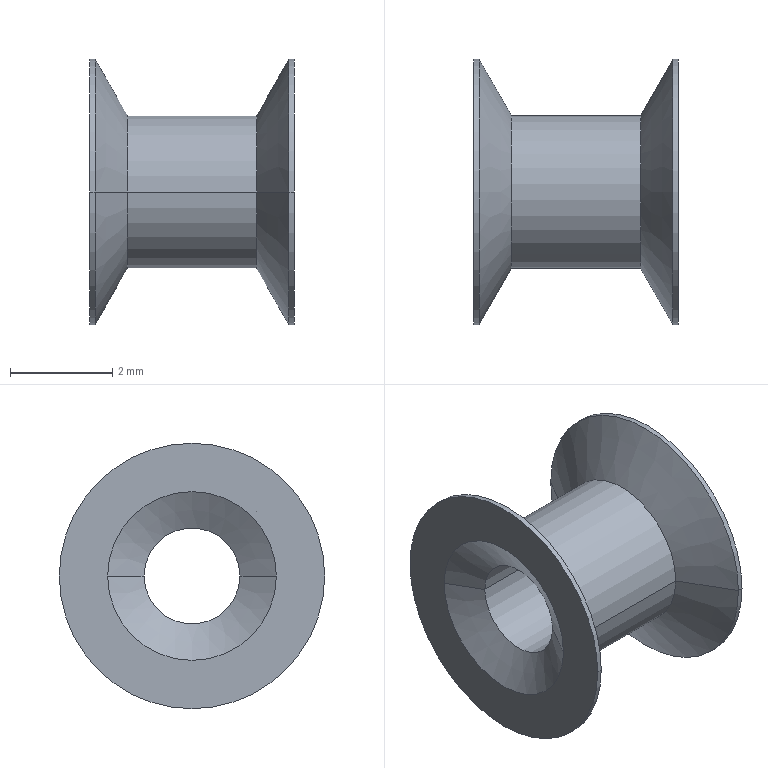Part | NX | features solid 2 | 1 solid | 18 faces | box 4 x 5.2 x 5.2 mm | volume 26.025 mm3 | cylinder 8 | cone 8 | plane 2 | commonest cylinder face diameters 5.2 x4 1.88 x2 3 x2
STEP:
#1=CARTESIAN_POINT('',(13.5,2156.1,-1040.27));
#2=VERTEX_POINT('',#1);
#3=CARTESIAN_POINT('',(13.5,2150.9,-1040.27));
#4=VERTEX_POINT('',#3);
#5=CARTESIAN_POINT('',(13.5,2153.5,-1040.27));
#6=DIRECTION('',(1.,0.,0.));
#7=DIRECTION('',(0.,1.,0.));
#8=AXIS2_PLACEMENT_3D('',#5,#6,#7);
#9=CIRCLE('',#8,2.6);
#10=EDGE_CURVE('',#2,#4,#9,.T.);
#11=ORIENTED_EDGE('',*,*,#10,.F.);
#12=CARTESIAN_POINT('',(13.5,2153.5,-1040.27));
#13=DIRECTION('',(1.,0.,0.));
#14=DIRECTION('',(0.,-1.,0.));
#15=AXIS2_PLACEMENT_3D('',#12,#13,#14);
#16=CIRCLE('',#15,2.6);
#17=EDGE_CURVE('',#4,#2,#16,.T.);
#18=ORIENTED_EDGE('',*,*,#17,.F.);
#19=EDGE_LOOP('',(#11,#18));
#20=FACE_BOUND('',#19,.T.);
#21=CARTESIAN_POINT('',(13.5,2155.153,-1040.27));
#22=VERTEX_POINT('',#21);
#23=CARTESIAN_POINT('',(13.5,2151.847,-1040.27));
#24=VERTEX_POINT('',#23);
#25=CARTESIAN_POINT('',(13.5,2153.5,-1040.27));
#26=DIRECTION('',(-1.,0.,0.));
#27=DIRECTION('',(0.,1.,0.));
#28=AXIS2_PLACEMENT_3D('',#25,#26,#27);
#29=CIRCLE('',#28,1.653);
#30=EDGE_CURVE('',#22,#24,#29,.T.);
#31=ORIENTED_EDGE('',*,*,#30,.F.);
#32=CARTESIAN_POINT('',(13.5,2153.5,-1040.27));
#33=DIRECTION('',(-1.,0.,0.));
#34=DIRECTION('',(0.,-1.,0.));
#35=AXIS2_PLACEMENT_3D('',#32,#33,#34);
#36=CIRCLE('',#35,1.653);
#37=EDGE_CURVE('',#24,#22,#36,.T.);
#38=ORIENTED_EDGE('',*,*,#37,.F.);
#39=EDGE_LOOP('',(#31,#38));
#40=FACE_BOUND('',#39,.T.);
#41=CARTESIAN_POINT('',(13.5,2153.5,-1040.27));
#42=DIRECTION('',(-1.,0.,0.));
#43=DIRECTION('',(0.,-1.,0.));
#44=AXIS2_PLACEMENT_3D('',#41,#42,#43);
#45=PLANE('',#44);
#46=ADVANCED_FACE('',(#20,#40),#45,.T.);
#47=ORIENTED_EDGE('',*,*,#17,.T.);
#48=CARTESIAN_POINT('',(13.6,2156.1,-1040.27));
#49=VERTEX_POINT('',#48);
#50=CARTESIAN_POINT('',(13.5,2156.1,-1040.27));
#51=DIRECTION('',(1.,0.,0.));
#52=VECTOR('',#51,1000.);
#53=LINE('',#50,#52);
#54=EDGE_CURVE('',#2,#49,#53,.T.);
#55=ORIENTED_EDGE('',*,*,#54,.T.);
#56=CARTESIAN_POINT('',(13.6,2150.9,-1040.27));
#57=VERTEX_POINT('',#56);
#58=CARTESIAN_POINT('',(13.6,2153.5,-1040.27));
#59=DIRECTION('',(-1.,0.,0.));
#60=DIRECTION('',(0.,1.,0.));
#61=AXIS2_PLACEMENT_3D('',#58,#59,#60);
#62=CIRCLE('',#61,2.6);
#63=EDGE_CURVE('',#49,#57,#62,.T.);
#64=ORIENTED_EDGE('',*,*,#63,.T.);
#65=CARTESIAN_POINT('',(13.5,2150.9,-1040.27));
#66=DIRECTION('',(1.,0.,0.));
#67=VECTOR('',#66,1000.);
#68=LINE('',#65,#67);
#69=EDGE_CURVE('',#57,#4,#68,.F.);
#70=ORIENTED_EDGE('',*,*,#69,.T.);
#71=EDGE_LOOP('',(#47,#55,#64,#70));
#72=FACE_BOUND('',#71,.T.);
#73=CARTESIAN_POINT('',(17.7,2153.5,-1040.27));
#74=DIRECTION('',(-1.,0.,0.));
#75=DIRECTION('',(0.,-1.,0.));
#76=AXIS2_PLACEMENT_3D('',#73,#74,#75);
#77=CYLINDRICAL_SURFACE('',#76,2.6);
#78=ADVANCED_FACE('',(#72),#77,.T.);
#79=CARTESIAN_POINT('',(13.6,2153.5,-1040.27));
#80=DIRECTION('',(-1.,0.,0.));
#81=DIRECTION('',(0.,-1.,0.));
#82=AXIS2_PLACEMENT_3D('',#79,#80,#81);
#83=CIRCLE('',#82,2.6);
#84=EDGE_CURVE('',#57,#49,#83,.T.);
#85=ORIENTED_EDGE('',*,*,#84,.T.);
#86=ORIENTED_EDGE('',*,*,#54,.F.);
#87=ORIENTED_EDGE('',*,*,#10,.T.);
#88=ORIENTED_EDGE('',*,*,#69,.F.);
#89=EDGE_LOOP('',(#85,#86,#87,#88));
#90=FACE_BOUND('',#89,.T.);
#91=CARTESIAN_POINT('',(17.7,2153.5,-1040.27));
#92=DIRECTION('',(-1.,0.,0.));
#93=DIRECTION('',(0.,-1.,0.));
#94=AXIS2_PLACEMENT_3D('',#91,#92,#93);
#95=CYLINDRICAL_SURFACE('',#94,2.6);
#96=ADVANCED_FACE('',(#90),#95,.T.);
#97=CARTESIAN_POINT('',(14.235,2155.,-1040.27));
#98=VERTEX_POINT('',#97);
#99=CARTESIAN_POINT('',(14.235,2152.,-1040.27));
#100=VERTEX_POINT('',#99);
#101=CARTESIAN_POINT('',(14.235,2153.5,-1040.27));
#102=DIRECTION('',(1.,0.,0.));
#103=DIRECTION('',(0.,1.,0.));
#104=AXIS2_PLACEMENT_3D('',#101,#102,#103);
#105=CIRCLE('',#104,1.5);
#106=EDGE_CURVE('',#98,#100,#105,.T.);
#107=ORIENTED_EDGE('',*,*,#106,.F.);
#108=CARTESIAN_POINT('',(13.6,2156.1,-1040.27));
#109=DIRECTION('',(0.5,-0.866,0.));
#110=VECTOR('',#109,1000.);
#111=LINE('',#108,#110);
#112=EDGE_CURVE('',#49,#98,#111,.T.);
#113=ORIENTED_EDGE('',*,*,#112,.F.);
#114=ORIENTED_EDGE('',*,*,#84,.F.);
#115=CARTESIAN_POINT('',(13.6,2150.9,-1040.27));
#116=DIRECTION('',(0.5,0.866,0.));
#117=VECTOR('',#116,1000.);
#118=LINE('',#115,#117);
#119=EDGE_CURVE('',#100,#57,#118,.F.);
#120=ORIENTED_EDGE('',*,*,#119,.F.);
#121=EDGE_LOOP('',(#107,#113,#114,#120));
#122=FACE_BOUND('',#121,.T.);
#123=CARTESIAN_POINT('',(13.918,2153.5,-1040.27));
#124=DIRECTION('',(-1.,0.,0.));
#125=DIRECTION('',(0.,-1.,0.));
#126=AXIS2_PLACEMENT_3D('',#123,#124,#125);
#127=CONICAL_SURFACE('',#126,2.05,1.047);
#128=ADVANCED_FACE('',(#122),#127,.T.);
#129=ORIENTED_EDGE('',*,*,#63,.F.);
#130=ORIENTED_EDGE('',*,*,#112,.T.);
#131=CARTESIAN_POINT('',(14.235,2153.5,-1040.27));
#132=DIRECTION('',(1.,0.,0.));
#133=DIRECTION('',(0.,-1.,0.));
#134=AXIS2_PLACEMENT_3D('',#131,#132,#133);
#135=CIRCLE('',#134,1.5);
#136=EDGE_CURVE('',#100,#98,#135,.T.);
#137=ORIENTED_EDGE('',*,*,#136,.F.);
#138=ORIENTED_EDGE('',*,*,#119,.T.);
#139=EDGE_LOOP('',(#129,#130,#137,#138));
#140=FACE_BOUND('',#139,.T.);
#141=CARTESIAN_POINT('',(13.918,2153.5,-1040.27));
#142=DIRECTION('',(-1.,0.,0.));
#143=DIRECTION('',(0.,-1.,0.));
#144=AXIS2_PLACEMENT_3D('',#141,#142,#143);
#145=CONICAL_SURFACE('',#144,2.05,1.047);
#146=ADVANCED_FACE('',(#140),#145,.T.);
#147=ORIENTED_EDGE('',*,*,#136,.T.);
#148=CARTESIAN_POINT('',(16.765,2155.,-1040.27));
#149=VERTEX_POINT('',#148);
#150=CARTESIAN_POINT('',(14.235,2155.,-1040.27));
#151=DIRECTION('',(1.,0.,0.));
#152=VECTOR('',#151,1000.);
#153=LINE('',#150,#152);
#154=EDGE_CURVE('',#98,#149,#153,.T.);
#155=ORIENTED_EDGE('',*,*,#154,.T.);
#156=CARTESIAN_POINT('',(16.765,2152.,-1040.27));
#157=VERTEX_POINT('',#156);
#158=CARTESIAN_POINT('',(16.765,2153.5,-1040.27));
#159=DIRECTION('',(-1.,0.,0.));
#160=DIRECTION('',(0.,1.,0.));
#161=AXIS2_PLACEMENT_3D('',#158,#159,#160);
#162=CIRCLE('',#161,1.5);
#163=EDGE_CURVE('',#149,#157,#162,.T.);
#164=ORIENTED_EDGE('',*,*,#163,.T.);
#165=CARTESIAN_POINT('',(14.235,2152.,-1040.27));
#166=DIRECTION('',(1.,0.,0.));
#167=VECTOR('',#166,1000.);
#168=LINE('',#165,#167);
#169=EDGE_CURVE('',#157,#100,#168,.F.);
#170=ORIENTED_EDGE('',*,*,#169,.T.);
#171=EDGE_LOOP('',(#147,#155,#164,#170));
#172=FACE_BOUND('',#171,.T.);
#173=CARTESIAN_POINT('',(17.7,2153.5,-1040.27));
#174=DIRECTION('',(-1.,0.,0.));
#175=DIRECTION('',(0.,-1.,0.));
#176=AXIS2_PLACEMENT_3D('',#173,#174,#175);
#177=CYLINDRICAL_SURFACE('',#176,1.5);
#178=ADVANCED_FACE('',(#172),#177,.T.);
#179=CARTESIAN_POINT('',(16.765,2153.5,-1040.27));
#180=DIRECTION('',(-1.,0.,0.));
#181=DIRECTION('',(0.,-1.,0.));
#182=AXIS2_PLACEMENT_3D('',#179,#180,#181);
#183=CIRCLE('',#182,1.5);
#184=EDGE_CURVE('',#157,#149,#183,.T.);
#185=ORIENTED_EDGE('',*,*,#184,.T.);
#186=ORIENTED_EDGE('',*,*,#154,.F.);
#187=ORIENTED_EDGE('',*,*,#106,.T.);
#188=ORIENTED_EDGE('',*,*,#169,.F.);
#189=EDGE_LOOP('',(#185,#186,#187,#188));
#190=FACE_BOUND('',#189,.T.);
#191=CARTESIAN_POINT('',(17.7,2153.5,-1040.27));
#192=DIRECTION('',(-1.,0.,0.));
#193=DIRECTION('',(0.,-1.,0.));
#194=AXIS2_PLACEMENT_3D('',#191,#192,#193);
#195=CYLINDRICAL_SURFACE('',#194,1.5);
#196=ADVANCED_FACE('',(#190),#195,.T.);
#197=CARTESIAN_POINT('',(17.4,2156.1,-1040.27));
#198=VERTEX_POINT('',#197);
#199=CARTESIAN_POINT('',(17.4,2150.9,-1040.27));
#200=VERTEX_POINT('',#199);
#201=CARTESIAN_POINT('',(17.4,2153.5,-1040.27));
#202=DIRECTION('',(1.,0.,0.));
#203=DIRECTION('',(0.,1.,0.));
#204=AXIS2_PLACEMENT_3D('',#201,#202,#203);
#205=CIRCLE('',#204,2.6);
#206=EDGE_CURVE('',#198,#200,#205,.T.);
#207=ORIENTED_EDGE('',*,*,#206,.F.);
#208=CARTESIAN_POINT('',(16.765,2155.,-1040.27));
#209=DIRECTION('',(0.5,0.866,0.));
#210=VECTOR('',#209,1000.);
#211=LINE('',#208,#210);
#212=EDGE_CURVE('',#149,#198,#211,.T.);
#213=ORIENTED_EDGE('',*,*,#212,.F.);
#214=ORIENTED_EDGE('',*,*,#184,.F.);
#215=CARTESIAN_POINT('',(16.765,2152.,-1040.27));
#216=DIRECTION('',(0.5,-0.866,0.));
#217=VECTOR('',#216,1000.);
#218=LINE('',#215,#217);
#219=EDGE_CURVE('',#200,#157,#218,.F.);
#220=ORIENTED_EDGE('',*,*,#219,.F.);
#221=EDGE_LOOP('',(#207,#213,#214,#220));
#222=FACE_BOUND('',#221,.T.);
#223=CARTESIAN_POINT('',(17.082,2153.5,-1040.27));
#224=DIRECTION('',(1.,0.,0.));
#225=DIRECTION('',(0.,1.,0.));
#226=AXIS2_PLACEMENT_3D('',#223,#224,#225);
#227=CONICAL_SURFACE('',#226,2.05,1.047);
#228=ADVANCED_FACE('',(#222),#227,.T.);
#229=ORIENTED_EDGE('',*,*,#163,.F.);
#230=ORIENTED_EDGE('',*,*,#212,.T.);
#231=CARTESIAN_POINT('',(17.4,2153.5,-1040.27));
#232=DIRECTION('',(1.,0.,0.));
#233=DIRECTION('',(0.,-1.,0.));
#234=AXIS2_PLACEMENT_3D('',#231,#232,#233);
#235=CIRCLE('',#234,2.6);
#236=EDGE_CURVE('',#200,#198,#235,.T.);
#237=ORIENTED_EDGE('',*,*,#236,.F.);
#238=ORIENTED_EDGE('',*,*,#219,.T.);
#239=EDGE_LOOP('',(#229,#230,#237,#238));
#240=FACE_BOUND('',#239,.T.);
#241=CARTESIAN_POINT('',(17.082,2153.5,-1040.27));
#242=DIRECTION('',(1.,0.,0.));
#243=DIRECTION('',(0.,1.,0.));
#244=AXIS2_PLACEMENT_3D('',#241,#242,#243);
#245=CONICAL_SURFACE('',#244,2.05,1.047);
#246=ADVANCED_FACE('',(#240),#245,.T.);
#247=ORIENTED_EDGE('',*,*,#236,.T.);
#248=CARTESIAN_POINT('',(17.5,2156.1,-1040.27));
#249=VERTEX_POINT('',#248);
#250=CARTESIAN_POINT('',(17.4,2156.1,-1040.27));
#251=DIRECTION('',(1.,0.,0.));
#252=VECTOR('',#251,1000.);
#253=LINE('',#250,#252);
#254=EDGE_CURVE('',#198,#249,#253,.T.);
#255=ORIENTED_EDGE('',*,*,#254,.T.);
#256=CARTESIAN_POINT('',(17.5,2150.9,-1040.27));
#257=VERTEX_POINT('',#256);
#258=CARTESIAN_POINT('',(17.5,2153.5,-1040.27));
#259=DIRECTION('',(-1.,0.,0.));
#260=DIRECTION('',(0.,1.,0.));
#261=AXIS2_PLACEMENT_3D('',#258,#259,#260);
#262=CIRCLE('',#261,2.6);
#263=EDGE_CURVE('',#249,#257,#262,.T.);
#264=ORIENTED_EDGE('',*,*,#263,.T.);
#265=CARTESIAN_POINT('',(17.4,2150.9,-1040.27));
#266=DIRECTION('',(1.,0.,0.));
#267=VECTOR('',#266,1000.);
#268=LINE('',#265,#267);
#269=EDGE_CURVE('',#257,#200,#268,.F.);
#270=ORIENTED_EDGE('',*,*,#269,.T.);
#271=EDGE_LOOP('',(#247,#255,#264,#270));
#272=FACE_BOUND('',#271,.T.);
#273=CARTESIAN_POINT('',(17.7,2153.5,-1040.27));
#274=DIRECTION('',(-1.,0.,0.));
#275=DIRECTION('',(0.,-1.,0.));
#276=AXIS2_PLACEMENT_3D('',#273,#274,#275);
#277=CYLINDRICAL_SURFACE('',#276,2.6);
#278=ADVANCED_FACE('',(#272),#277,.T.);
#279=CARTESIAN_POINT('',(17.5,2153.5,-1040.27));
#280=DIRECTION('',(-1.,0.,0.));
#281=DIRECTION('',(0.,-1.,0.));
#282=AXIS2_PLACEMENT_3D('',#279,#280,#281);
#283=CIRCLE('',#282,2.6);
#284=EDGE_CURVE('',#257,#249,#283,.T.);
#285=ORIENTED_EDGE('',*,*,#284,.T.);
#286=ORIENTED_EDGE('',*,*,#254,.F.);
#287=ORIENTED_EDGE('',*,*,#206,.T.);
#288=ORIENTED_EDGE('',*,*,#269,.F.);
#289=EDGE_LOOP('',(#285,#286,#287,#288));
#290=FACE_BOUND('',#289,.T.);
#291=CARTESIAN_POINT('',(17.7,2153.5,-1040.27));
#292=DIRECTION('',(-1.,0.,0.));
#293=DIRECTION('',(0.,-1.,0.));
#294=AXIS2_PLACEMENT_3D('',#291,#292,#293);
#295=CYLINDRICAL_SURFACE('',#294,2.6);
#296=ADVANCED_FACE('',(#290),#295,.T.);
#297=ORIENTED_EDGE('',*,*,#284,.F.);
#298=ORIENTED_EDGE('',*,*,#263,.F.);
#299=EDGE_LOOP('',(#297,#298));
#300=FACE_BOUND('',#299,.T.);
#301=CARTESIAN_POINT('',(17.5,2151.847,-1040.27));
#302=VERTEX_POINT('',#301);
#303=CARTESIAN_POINT('',(17.5,2155.153,-1040.27));
#304=VERTEX_POINT('',#303);
#305=CARTESIAN_POINT('',(17.5,2153.5,-1040.27));
#306=DIRECTION('',(1.,0.,0.));
#307=DIRECTION('',(0.,-1.,0.));
#308=AXIS2_PLACEMENT_3D('',#305,#306,#307);
#309=CIRCLE('',#308,1.653);
#310=EDGE_CURVE('',#302,#304,#309,.T.);
#311=ORIENTED_EDGE('',*,*,#310,.F.);
#312=CARTESIAN_POINT('',(17.5,2153.5,-1040.27));
#313=DIRECTION('',(1.,0.,0.));
#314=DIRECTION('',(0.,1.,0.));
#315=AXIS2_PLACEMENT_3D('',#312,#313,#314);
#316=CIRCLE('',#315,1.653);
#317=EDGE_CURVE('',#304,#302,#316,.T.);
#318=ORIENTED_EDGE('',*,*,#317,.F.);
#319=EDGE_LOOP('',(#311,#318));
#320=FACE_BOUND('',#319,.T.);
#321=CARTESIAN_POINT('',(17.5,2153.5,-1040.27));
#322=DIRECTION('',(-1.,0.,0.));
#323=DIRECTION('',(0.,-1.,0.));
#324=AXIS2_PLACEMENT_3D('',#321,#322,#323);
#325=PLANE('',#324);
#326=ADVANCED_FACE('',(#300,#320),#325,.F.);
#327=CARTESIAN_POINT('',(17.088,2152.56,-1040.27));
#328=VERTEX_POINT('',#327);
#329=CARTESIAN_POINT('',(17.088,2152.56,-1040.27));
#330=DIRECTION('',(0.5,-0.866,0.));
#331=VECTOR('',#330,1000.);
#332=LINE('',#329,#331);
#333=EDGE_CURVE('',#328,#302,#332,.T.);
#334=ORIENTED_EDGE('',*,*,#333,.F.);
#335=CARTESIAN_POINT('',(17.088,2154.44,-1040.27));
#336=VERTEX_POINT('',#335);
#337=CARTESIAN_POINT('',(17.088,2153.5,-1040.27));
#338=DIRECTION('',(1.,0.,0.));
#339=DIRECTION('',(0.,1.,0.));
#340=AXIS2_PLACEMENT_3D('',#337,#338,#339);
#341=CIRCLE('',#340,0.94);
#342=EDGE_CURVE('',#336,#328,#341,.T.);
#343=ORIENTED_EDGE('',*,*,#342,.F.);
#344=CARTESIAN_POINT('',(17.088,2154.44,-1040.27));
#345=DIRECTION('',(0.5,0.866,0.));
#346=VECTOR('',#345,1000.);
#347=LINE('',#344,#346);
#348=EDGE_CURVE('',#304,#336,#347,.F.);
#349=ORIENTED_EDGE('',*,*,#348,.F.);
#350=ORIENTED_EDGE('',*,*,#317,.T.);
#351=EDGE_LOOP('',(#334,#343,#349,#350));
#352=FACE_BOUND('',#351,.T.);
#353=CARTESIAN_POINT('',(17.294,2153.5,-1040.27));
#354=DIRECTION('',(1.,0.,0.));
#355=DIRECTION('',(0.,1.,0.));
#356=AXIS2_PLACEMENT_3D('',#353,#354,#355);
#357=CONICAL_SURFACE('',#356,1.297,1.047);
#358=ADVANCED_FACE('',(#352),#357,.F.);
#359=ORIENTED_EDGE('',*,*,#348,.T.);
#360=CARTESIAN_POINT('',(17.088,2153.5,-1040.27));
#361=DIRECTION('',(1.,0.,0.));
#362=DIRECTION('',(0.,-1.,0.));
#363=AXIS2_PLACEMENT_3D('',#360,#361,#362);
#364=CIRCLE('',#363,0.94);
#365=EDGE_CURVE('',#328,#336,#364,.T.);
#366=ORIENTED_EDGE('',*,*,#365,.F.);
#367=ORIENTED_EDGE('',*,*,#333,.T.);
#368=ORIENTED_EDGE('',*,*,#310,.T.);
#369=EDGE_LOOP('',(#359,#366,#367,#368));
#370=FACE_BOUND('',#369,.T.);
#371=CARTESIAN_POINT('',(17.294,2153.5,-1040.27));
#372=DIRECTION('',(1.,0.,0.));
#373=DIRECTION('',(0.,1.,0.));
#374=AXIS2_PLACEMENT_3D('',#371,#372,#373);
#375=CONICAL_SURFACE('',#374,1.297,1.047);
#376=ADVANCED_FACE('',(#370),#375,.F.);
#377=ORIENTED_EDGE('',*,*,#365,.T.);
#378=CARTESIAN_POINT('',(13.912,2154.44,-1040.27));
#379=VERTEX_POINT('',#378);
#380=CARTESIAN_POINT('',(13.912,2154.44,-1040.27));
#381=DIRECTION('',(1.,0.,0.));
#382=VECTOR('',#381,1000.);
#383=LINE('',#380,#382);
#384=EDGE_CURVE('',#336,#379,#383,.F.);
#385=ORIENTED_EDGE('',*,*,#384,.T.);
#386=CARTESIAN_POINT('',(13.912,2152.56,-1040.27));
#387=VERTEX_POINT('',#386);
#388=CARTESIAN_POINT('',(13.912,2153.5,-1040.27));
#389=DIRECTION('',(-1.,0.,0.));
#390=DIRECTION('',(0.,1.,0.));
#391=AXIS2_PLACEMENT_3D('',#388,#389,#390);
#392=CIRCLE('',#391,0.94);
#393=EDGE_CURVE('',#379,#387,#392,.T.);
#394=ORIENTED_EDGE('',*,*,#393,.T.);
#395=CARTESIAN_POINT('',(13.912,2152.56,-1040.27));
#396=DIRECTION('',(1.,0.,0.));
#397=VECTOR('',#396,1000.);
#398=LINE('',#395,#397);
#399=EDGE_CURVE('',#387,#328,#398,.T.);
#400=ORIENTED_EDGE('',*,*,#399,.T.);
#401=EDGE_LOOP('',(#377,#385,#394,#400));
#402=FACE_BOUND('',#401,.T.);
#403=CARTESIAN_POINT('',(17.7,2153.5,-1040.27));
#404=DIRECTION('',(-1.,0.,0.));
#405=DIRECTION('',(0.,-1.,0.));
#406=AXIS2_PLACEMENT_3D('',#403,#404,#405);
#407=CYLINDRICAL_SURFACE('',#406,0.94);
#408=ADVANCED_FACE('',(#402),#407,.F.);
#409=CARTESIAN_POINT('',(13.912,2153.5,-1040.27));
#410=DIRECTION('',(-1.,0.,0.));
#411=DIRECTION('',(0.,-1.,0.));
#412=AXIS2_PLACEMENT_3D('',#409,#410,#411);
#413=CIRCLE('',#412,0.94);
#414=EDGE_CURVE('',#387,#379,#413,.T.);
#415=ORIENTED_EDGE('',*,*,#414,.T.);
#416=ORIENTED_EDGE('',*,*,#384,.F.);
#417=ORIENTED_EDGE('',*,*,#342,.T.);
#418=ORIENTED_EDGE('',*,*,#399,.F.);
#419=EDGE_LOOP('',(#415,#416,#417,#418));
#420=FACE_BOUND('',#419,.T.);
#421=CARTESIAN_POINT('',(17.7,2153.5,-1040.27));
#422=DIRECTION('',(-1.,0.,0.));
#423=DIRECTION('',(0.,-1.,0.));
#424=AXIS2_PLACEMENT_3D('',#421,#422,#423);
#425=CYLINDRICAL_SURFACE('',#424,0.94);
#426=ADVANCED_FACE('',(#420),#425,.F.);
#427=CARTESIAN_POINT('',(13.5,2155.153,-1040.27));
#428=DIRECTION('',(0.5,-0.866,0.));
#429=VECTOR('',#428,1000.);
#430=LINE('',#427,#429);
#431=EDGE_CURVE('',#379,#22,#430,.F.);
#432=ORIENTED_EDGE('',*,*,#431,.F.);
#433=ORIENTED_EDGE('',*,*,#414,.F.);
#434=CARTESIAN_POINT('',(13.5,2151.847,-1040.27));
#435=DIRECTION('',(0.5,0.866,0.));
#436=VECTOR('',#435,1000.);
#437=LINE('',#434,#436);
#438=EDGE_CURVE('',#24,#387,#437,.T.);
#439=ORIENTED_EDGE('',*,*,#438,.F.);
#440=ORIENTED_EDGE('',*,*,#37,.T.);
#441=EDGE_LOOP('',(#432,#433,#439,#440));
#442=FACE_BOUND('',#441,.T.);
#443=CARTESIAN_POINT('',(13.706,2153.5,-1040.27));
#444=DIRECTION('',(-1.,0.,0.));
#445=DIRECTION('',(0.,-1.,0.));
#446=AXIS2_PLACEMENT_3D('',#443,#444,#445);
#447=CONICAL_SURFACE('',#446,1.297,1.047);
#448=ADVANCED_FACE('',(#442),#447,.F.);
#449=ORIENTED_EDGE('',*,*,#438,.T.);
#450=ORIENTED_EDGE('',*,*,#393,.F.);
#451=ORIENTED_EDGE('',*,*,#431,.T.);
#452=ORIENTED_EDGE('',*,*,#30,.T.);
#453=EDGE_LOOP('',(#449,#450,#451,#452));
#454=FACE_BOUND('',#453,.T.);
#455=CARTESIAN_POINT('',(13.706,2153.5,-1040.27));
#456=DIRECTION('',(-1.,0.,0.));
#457=DIRECTION('',(0.,-1.,0.));
#458=AXIS2_PLACEMENT_3D('',#455,#456,#457);
#459=CONICAL_SURFACE('',#458,1.297,1.047);
#460=ADVANCED_FACE('',(#454),#459,.F.);
#461=CLOSED_SHELL('',(#46,#78,#96,#128,#146,#178,#196,#228,#246,#278,#296,#326,#358,#376,#408,#426,#448,#460));
#462=MANIFOLD_SOLID_BREP('',#461);
#463=(LENGTH_UNIT()NAMED_UNIT(*)SI_UNIT(.MILLI.,.METRE.));
#464=UNCERTAINTY_MEASURE_WITH_UNIT(LENGTH_MEASURE(0.00001),#463,'','');
#465=(NAMED_UNIT(*)PLANE_ANGLE_UNIT()SI_UNIT($,.RADIAN.));
#466=(NAMED_UNIT(*)SI_UNIT($,.STERADIAN.)SOLID_ANGLE_UNIT());
#467=(GEOMETRIC_REPRESENTATION_CONTEXT(3)GLOBAL_UNCERTAINTY_ASSIGNED_CONTEXT((#464))GLOBAL_UNIT_ASSIGNED_CONTEXT((#463,#465,#466))REPRESENTATION_CONTEXT('',''));
#468=ADVANCED_BREP_SHAPE_REPRESENTATION('',(#462),#467);